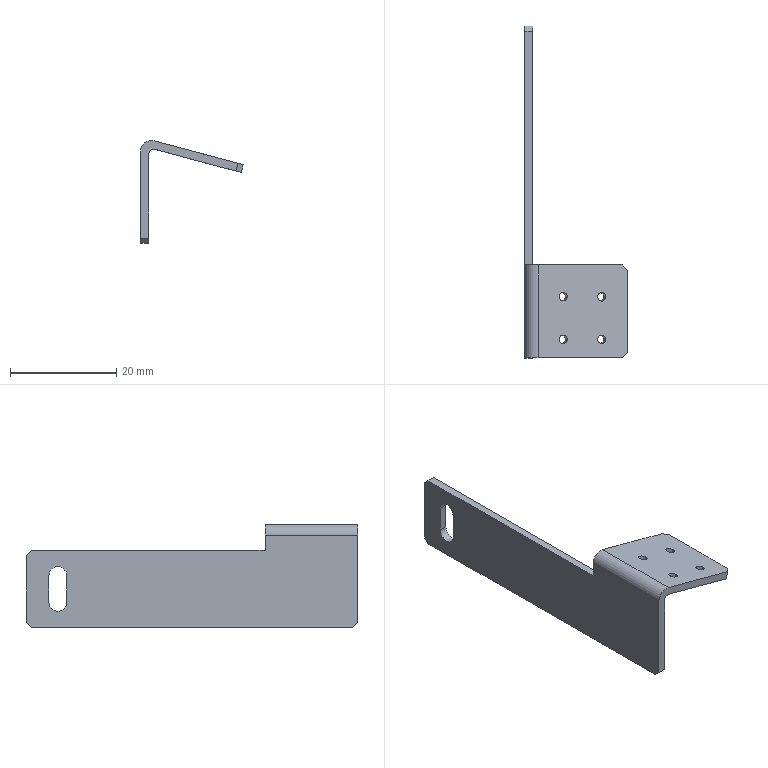Part | STEP file | PN_0014 | 1 solid | 31 faces | box 19.319 x 62.5 x 19.394 mm | volume 1902 mm3 | plane 17 | cylinder 14 | commonest cylinder face diameters 1.6 x8 3.4 x3 2 x2 4 x1